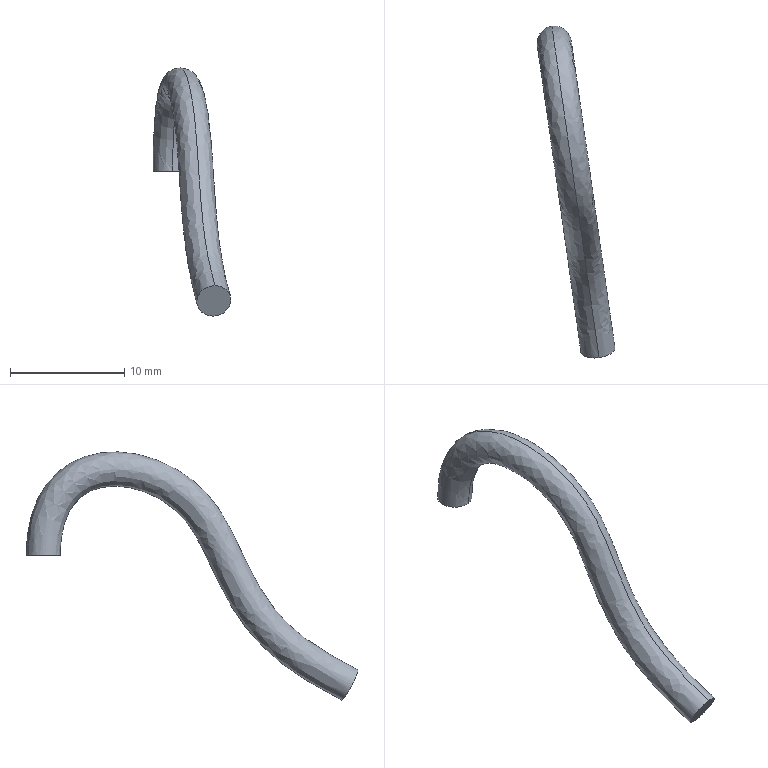Part | STEP file | MSBR-6_1_1_1_1 | 1 solid | 4 faces | box 6.81 x 29.042 x 21.733 mm | volume 286.346 mm3 | plane 2 | spline 2